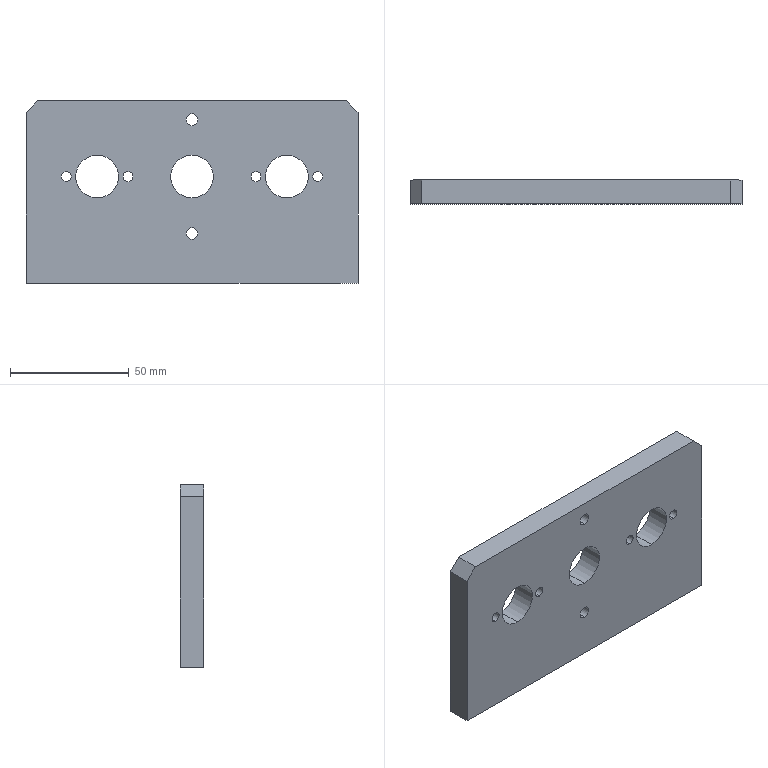Part | STEP file | 0232_203_Plate | 1 solid | 42 faces | box 140 x 10 x 77 mm | volume 97359 mm3 | cylinder 26 | cone 8 | plane 8 | commonest cylinder face diameters 5 x12 4.2 x8 18 x6